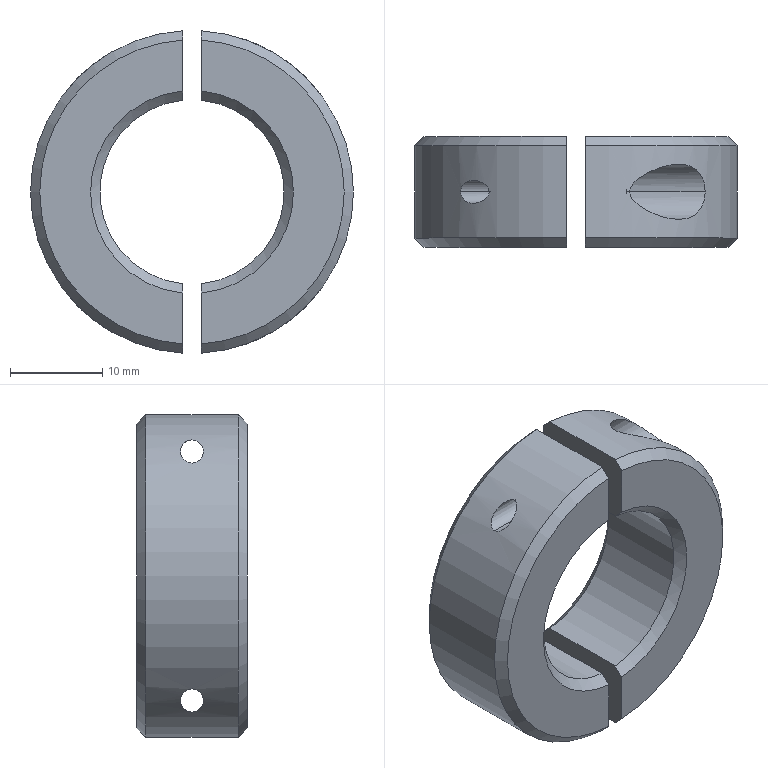Part | SolidWorks | features HoleWzd 2, Chamfer 1, Extrusion 1, ICE 1, MirrorPattern 1 | 2 solids | 34 faces | box 35 x 12 x 34.943 mm | volume 6766 mm3 | cylinder 16 | plane 10 | cone 8 | commonest cylinder face diameters 2.5 x4 3.4 x4 6 x4 20 x2 35 x2
STEP:
#1=CARTESIAN_POINT('',(1.,0.,11.8));
#2=VERTEX_POINT('',#1);
#3=CARTESIAN_POINT('',(1.,0.,15.2));
#4=VERTEX_POINT('',#3);
#5=CARTESIAN_POINT('',(1.,0.,13.5));
#6=DIRECTION('',(1.,0.,0.));
#7=DIRECTION('',(0.,0.,1.));
#8=AXIS2_PLACEMENT_3D('',#5,#6,#7);
#9=CIRCLE('',#8,1.7);
#10=EDGE_CURVE('',#2,#4,#9,.T.);
#11=ORIENTED_EDGE('',*,*,#10,.F.);
#12=CARTESIAN_POINT('',(5.5,0.,11.8));
#13=VERTEX_POINT('',#12);
#14=CARTESIAN_POINT('',(17.5,0.,11.8));
#15=DIRECTION('',(1.,0.,0.));
#16=VECTOR('',#15,1000.);
#17=LINE('',#14,#16);
#18=EDGE_CURVE('',#2,#13,#17,.T.);
#19=ORIENTED_EDGE('',*,*,#18,.T.);
#20=CARTESIAN_POINT('',(5.5,0.,15.2));
#21=VERTEX_POINT('',#20);
#22=CARTESIAN_POINT('',(5.5,0.,13.5));
#23=DIRECTION('',(-1.,0.,0.));
#24=DIRECTION('',(0.,0.,1.));
#25=AXIS2_PLACEMENT_3D('',#22,#23,#24);
#26=CIRCLE('',#25,1.7);
#27=EDGE_CURVE('',#21,#13,#26,.T.);
#28=ORIENTED_EDGE('',*,*,#27,.F.);
#29=CARTESIAN_POINT('',(17.5,0.,15.2));
#30=DIRECTION('',(1.,0.,0.));
#31=VECTOR('',#30,1000.);
#32=LINE('',#29,#31);
#33=EDGE_CURVE('',#4,#21,#32,.T.);
#34=ORIENTED_EDGE('',*,*,#33,.F.);
#35=EDGE_LOOP('',(#11,#19,#28,#34));
#36=FACE_OUTER_BOUND('',#35,.T.);
#37=CARTESIAN_POINT('',(17.5,0.,13.5));
#38=DIRECTION('',(1.,0.,0.));
#39=DIRECTION('',(0.,0.,1.));
#40=AXIS2_PLACEMENT_3D('',#37,#38,#39);
#41=CYLINDRICAL_SURFACE('',#40,1.7);
#42=ADVANCED_FACE('',(#36),#41,.F.);
#43=CARTESIAN_POINT('',(5.5,0.,16.5));
#44=VERTEX_POINT('',#43);
#45=CARTESIAN_POINT('',(5.5,0.,10.5));
#46=VERTEX_POINT('',#45);
#47=CARTESIAN_POINT('',(5.5,0.,13.5));
#48=DIRECTION('',(-1.,0.,0.));
#49=DIRECTION('',(0.,0.,1.));
#50=AXIS2_PLACEMENT_3D('',#47,#48,#49);
#51=CIRCLE('',#50,3.);
#52=EDGE_CURVE('',#44,#46,#51,.T.);
#53=ORIENTED_EDGE('',*,*,#52,.T.);
#54=CARTESIAN_POINT('',(14.,0.,10.5));
#55=VERTEX_POINT('',#54);
#56=CARTESIAN_POINT('',(17.5,0.,10.5));
#57=DIRECTION('',(1.,0.,0.));
#58=VECTOR('',#57,1000.);
#59=LINE('',#56,#58);
#60=EDGE_CURVE('',#46,#55,#59,.T.);
#61=ORIENTED_EDGE('',*,*,#60,.T.);
#62=CARTESIAN_POINT('',(5.831,0.,16.5));
#63=VERTEX_POINT('',#62);
#64=CARTESIAN_POINT('',(14.,0.,10.5));
#65=CARTESIAN_POINT('',(14.,0.273,10.5));
#66=CARTESIAN_POINT('',(13.973,0.5393,10.537));
#67=CARTESIAN_POINT('',(13.864,1.056,10.679));
#68=CARTESIAN_POINT('',(13.786,1.293,10.781));
#69=CARTESIAN_POINT('',(13.582,1.731,11.037));
#70=CARTESIAN_POINT('',(13.461,1.922,11.185));
#71=CARTESIAN_POINT('',(13.183,2.258,11.511));
#72=CARTESIAN_POINT('',(13.03,2.398,11.685));
#73=CARTESIAN_POINT('',(12.701,2.63,12.041));
#74=CARTESIAN_POINT('',(12.523,2.724,12.227));
#75=CARTESIAN_POINT('',(12.154,2.867,12.594));
#76=CARTESIAN_POINT('',(11.963,2.917,12.775));
#77=CARTESIAN_POINT('',(11.569,2.983,13.133));
#78=CARTESIAN_POINT('',(11.364,2.999,13.311));
#79=CARTESIAN_POINT('',(10.948,3.001,13.656));
#80=CARTESIAN_POINT('',(10.737,2.987,13.822));
#81=CARTESIAN_POINT('',(10.099,2.909,14.302));
#82=CARTESIAN_POINT('',(9.664,2.809,14.599));
#83=CARTESIAN_POINT('',(8.778,2.526,15.148));
#84=CARTESIAN_POINT('',(8.336,2.346,15.395));
#85=CARTESIAN_POINT('',(7.683,2.018,15.725));
#86=CARTESIAN_POINT('',(7.466,1.898,15.829));
#87=CARTESIAN_POINT('',(7.041,1.632,16.023));
#88=CARTESIAN_POINT('',(6.83,1.484,16.114));
#89=CARTESIAN_POINT('',(6.434,1.153,16.276));
#90=CARTESIAN_POINT('',(6.246,0.968,16.348));
#91=CARTESIAN_POINT('',(6.02,0.6436,16.432));
#92=CARTESIAN_POINT('',(5.953,0.5249,16.456));
#93=CARTESIAN_POINT('',(5.859,0.2731,16.49));
#94=CARTESIAN_POINT('',(5.831,0.1376,16.5));
#95=CARTESIAN_POINT('',(5.831,0.,16.5));
#96=B_SPLINE_CURVE_WITH_KNOTS('',3,(#64,#65,#66,#67,#68,#69,#70,#71,#72,#73,#74,#75,#76,#77,#78,#79,#80,#81,#82,#83,#84,#85,#86,#87,#88,#89,#90,#91,#92,#93,#94,#95),.UNSPECIFIED.,.F.,.F.,(4,2,2,2,2,2,2,2,2,2,2,2,2,2,2,4),(0.01297,0.01378,0.01459,0.0154,0.01621,0.01702,0.01783,0.01864,0.01945,0.02107,0.02269,0.02351,0.02432,0.02513,0.02553,0.02594),.UNSPECIFIED.);
#97=EDGE_CURVE('',#55,#63,#96,.T.);
#98=ORIENTED_EDGE('',*,*,#97,.T.);
#99=CARTESIAN_POINT('',(17.5,0.,16.5));
#100=DIRECTION('',(1.,0.,0.));
#101=VECTOR('',#100,1000.);
#102=LINE('',#99,#101);
#103=EDGE_CURVE('',#44,#63,#102,.T.);
#104=ORIENTED_EDGE('',*,*,#103,.F.);
#105=EDGE_LOOP('',(#53,#61,#98,#104));
#106=FACE_OUTER_BOUND('',#105,.T.);
#107=CARTESIAN_POINT('',(17.5,0.,13.5));
#108=DIRECTION('',(1.,0.,0.));
#109=DIRECTION('',(0.,0.,1.));
#110=AXIS2_PLACEMENT_3D('',#107,#108,#109);
#111=CYLINDRICAL_SURFACE('',#110,3.);
#112=ADVANCED_FACE('',(#106),#111,.F.);
#113=CARTESIAN_POINT('',(1.,0.,-15.2));
#114=VERTEX_POINT('',#113);
#115=CARTESIAN_POINT('',(1.,0.,-11.8));
#116=VERTEX_POINT('',#115);
#117=CARTESIAN_POINT('',(1.,0.,-13.5));
#118=DIRECTION('',(-1.,0.,0.));
#119=DIRECTION('',(0.,0.,-1.));
#120=AXIS2_PLACEMENT_3D('',#117,#118,#119);
#121=CIRCLE('',#120,1.7);
#122=EDGE_CURVE('',#114,#116,#121,.T.);
#123=ORIENTED_EDGE('',*,*,#122,.T.);
#124=CARTESIAN_POINT('',(5.5,0.,-11.8));
#125=VERTEX_POINT('',#124);
#126=CARTESIAN_POINT('',(17.5,0.,-11.8));
#127=DIRECTION('',(1.,0.,0.));
#128=VECTOR('',#127,1000.);
#129=LINE('',#126,#128);
#130=EDGE_CURVE('',#116,#125,#129,.T.);
#131=ORIENTED_EDGE('',*,*,#130,.T.);
#132=CARTESIAN_POINT('',(5.5,0.,-15.2));
#133=VERTEX_POINT('',#132);
#134=CARTESIAN_POINT('',(5.5,0.,-13.5));
#135=DIRECTION('',(1.,0.,0.));
#136=DIRECTION('',(0.,0.,-1.));
#137=AXIS2_PLACEMENT_3D('',#134,#135,#136);
#138=CIRCLE('',#137,1.7);
#139=EDGE_CURVE('',#125,#133,#138,.T.);
#140=ORIENTED_EDGE('',*,*,#139,.T.);
#141=CARTESIAN_POINT('',(17.5,0.,-15.2));
#142=DIRECTION('',(1.,0.,0.));
#143=VECTOR('',#142,1000.);
#144=LINE('',#141,#143);
#145=EDGE_CURVE('',#114,#133,#144,.T.);
#146=ORIENTED_EDGE('',*,*,#145,.F.);
#147=EDGE_LOOP('',(#123,#131,#140,#146));
#148=FACE_OUTER_BOUND('',#147,.T.);
#149=CARTESIAN_POINT('',(17.5,0.,-13.5));
#150=DIRECTION('',(1.,0.,0.));
#151=DIRECTION('',(0.,0.,-1.));
#152=AXIS2_PLACEMENT_3D('',#149,#150,#151);
#153=CYLINDRICAL_SURFACE('',#152,1.7);
#154=ADVANCED_FACE('',(#148),#153,.F.);
#155=CARTESIAN_POINT('',(5.5,0.,-10.5));
#156=VERTEX_POINT('',#155);
#157=CARTESIAN_POINT('',(5.5,0.,-16.5));
#158=VERTEX_POINT('',#157);
#159=CARTESIAN_POINT('',(5.5,0.,-13.5));
#160=DIRECTION('',(1.,0.,0.));
#161=DIRECTION('',(0.,0.,-1.));
#162=AXIS2_PLACEMENT_3D('',#159,#160,#161);
#163=CIRCLE('',#162,3.);
#164=EDGE_CURVE('',#156,#158,#163,.T.);
#165=ORIENTED_EDGE('',*,*,#164,.F.);
#166=CARTESIAN_POINT('',(14.,0.,-10.5));
#167=VERTEX_POINT('',#166);
#168=CARTESIAN_POINT('',(17.5,0.,-10.5));
#169=DIRECTION('',(1.,0.,0.));
#170=VECTOR('',#169,1000.);
#171=LINE('',#168,#170);
#172=EDGE_CURVE('',#156,#167,#171,.T.);
#173=ORIENTED_EDGE('',*,*,#172,.T.);
#174=CARTESIAN_POINT('',(5.831,0.,-16.5));
#175=VERTEX_POINT('',#174);
#176=CARTESIAN_POINT('',(5.831,0.,-16.5));
#177=CARTESIAN_POINT('',(5.831,-0.1376,-16.5));
#178=CARTESIAN_POINT('',(5.858,-0.2701,-16.491));
#179=CARTESIAN_POINT('',(5.953,-0.5249,-16.457));
#180=CARTESIAN_POINT('',(6.018,-0.641,-16.433));
#181=CARTESIAN_POINT('',(6.17,-0.8592,-16.377));
#182=CARTESIAN_POINT('',(6.256,-0.9603,-16.344));
#183=CARTESIAN_POINT('',(6.437,-1.148,-16.274));
#184=CARTESIAN_POINT('',(6.532,-1.235,-16.236));
#185=CARTESIAN_POINT('',(6.829,-1.483,-16.114));
#186=CARTESIAN_POINT('',(7.039,-1.631,-16.024));
#187=CARTESIAN_POINT('',(7.464,-1.897,-15.83));
#188=CARTESIAN_POINT('',(7.68,-2.017,-15.726));
#189=CARTESIAN_POINT('',(8.335,-2.346,-15.395));
#190=CARTESIAN_POINT('',(8.783,-2.527,-15.145));
#191=CARTESIAN_POINT('',(9.664,-2.808,-14.599));
#192=CARTESIAN_POINT('',(10.098,-2.909,-14.303));
#193=CARTESIAN_POINT('',(10.74,-2.987,-13.819));
#194=CARTESIAN_POINT('',(10.953,-3.001,-13.651));
#195=CARTESIAN_POINT('',(11.368,-2.999,-13.308));
#196=CARTESIAN_POINT('',(11.57,-2.983,-13.132));
#197=CARTESIAN_POINT('',(11.965,-2.916,-12.773));
#198=CARTESIAN_POINT('',(12.159,-2.865,-12.589));
#199=CARTESIAN_POINT('',(12.528,-2.721,-12.222));
#200=CARTESIAN_POINT('',(12.703,-2.629,-12.04));
#201=CARTESIAN_POINT('',(13.032,-2.396,-11.682));
#202=CARTESIAN_POINT('',(13.187,-2.253,-11.506));
#203=CARTESIAN_POINT('',(13.393,-2.004,-11.264));
#204=CARTESIAN_POINT('',(13.458,-1.914,-11.187));
#205=CARTESIAN_POINT('',(13.578,-1.722,-11.04));
#206=CARTESIAN_POINT('',(13.635,-1.618,-10.97));
#207=CARTESIAN_POINT('',(13.735,-1.401,-10.844));
#208=CARTESIAN_POINT('',(13.78,-1.287,-10.787));
#209=CARTESIAN_POINT('',(13.858,-1.049,-10.687));
#210=CARTESIAN_POINT('',(13.892,-0.9236,-10.643));
#211=CARTESIAN_POINT('',(13.973,-0.5391,-10.537));
#212=CARTESIAN_POINT('',(14.,-0.273,-10.5));
#213=CARTESIAN_POINT('',(14.,0.,-10.5));
#214=B_SPLINE_CURVE_WITH_KNOTS('',3,(#176,#177,#178,#179,#180,#181,#182,#183,#184,#185,#186,#187,#188,#189,#190,#191,#192,#193,#194,#195,#196,#197,#198,#199,#200,#201,#202,#203,#204,#205,#206,#207,#208,#209,#210,#211,#212,#213),.UNSPECIFIED.,.F.,.F.,(4,2,2,2,2,2,2,2,2,2,2,2,2,2,2,2,2,2,4),(0.,0.0004053,0.0008105,0.001216,0.001621,0.002432,0.003242,0.004863,0.006484,0.007295,0.008105,0.008916,0.009726,0.01054,0.01094,0.01135,0.01175,0.01216,0.01297),.UNSPECIFIED.);
#215=EDGE_CURVE('',#175,#167,#214,.T.);
#216=ORIENTED_EDGE('',*,*,#215,.F.);
#217=CARTESIAN_POINT('',(17.5,0.,-16.5));
#218=DIRECTION('',(1.,0.,0.));
#219=VECTOR('',#218,1000.);
#220=LINE('',#217,#219);
#221=EDGE_CURVE('',#158,#175,#220,.T.);
#222=ORIENTED_EDGE('',*,*,#221,.F.);
#223=EDGE_LOOP('',(#165,#173,#216,#222));
#224=FACE_OUTER_BOUND('',#223,.T.);
#225=CARTESIAN_POINT('',(17.5,0.,-13.5));
#226=DIRECTION('',(1.,0.,0.));
#227=DIRECTION('',(0.,0.,-1.));
#228=AXIS2_PLACEMENT_3D('',#225,#226,#227);
#229=CYLINDRICAL_SURFACE('',#228,3.);
#230=ADVANCED_FACE('',(#224),#229,.F.);
#231=CARTESIAN_POINT('',(1.,-6.,-10.954));
#232=VERTEX_POINT('',#231);
#233=CARTESIAN_POINT('',(1.,-5.,-9.95));
#234=VERTEX_POINT('',#233);
#235=CARTESIAN_POINT('',(1.,-6.,-10.954));
#236=CARTESIAN_POINT('',(1.,-5.667,-10.62));
#237=CARTESIAN_POINT('',(1.,-5.333,-10.285));
#238=CARTESIAN_POINT('',(1.,-5.,-9.95));
#239=B_SPLINE_CURVE_WITH_KNOTS('',3,(#235,#236,#237,#238),.UNSPECIFIED.,.F.,.F.,(4,4),(0.000000992,0.001418),.UNSPECIFIED.);
#240=EDGE_CURVE('',#232,#234,#239,.T.);
#241=ORIENTED_EDGE('',*,*,#240,.T.);
#242=CARTESIAN_POINT('',(1.,5.,-9.95));
#243=VERTEX_POINT('',#242);
#244=CARTESIAN_POINT('',(1.,6.,-9.95));
#245=DIRECTION('',(0.,1.,0.));
#246=VECTOR('',#245,1000.);
#247=LINE('',#244,#246);
#248=EDGE_CURVE('',#234,#243,#247,.T.);
#249=ORIENTED_EDGE('',*,*,#248,.T.);
#250=CARTESIAN_POINT('',(1.,6.,-10.954));
#251=VERTEX_POINT('',#250);
#252=CARTESIAN_POINT('',(1.,5.,-9.95));
#253=CARTESIAN_POINT('',(1.,5.333,-10.285));
#254=CARTESIAN_POINT('',(1.,5.667,-10.62));
#255=CARTESIAN_POINT('',(1.,6.,-10.954));
#256=B_SPLINE_CURVE_WITH_KNOTS('',3,(#252,#253,#254,#255),.UNSPECIFIED.,.F.,.F.,(4,4),(0.02841,0.02983),.UNSPECIFIED.);
#257=EDGE_CURVE('',#243,#251,#256,.T.);
#258=ORIENTED_EDGE('',*,*,#257,.T.);
#259=CARTESIAN_POINT('',(1.,6.,-16.47));
#260=VERTEX_POINT('',#259);
#261=CARTESIAN_POINT('',(1.,6.,20.));
#262=DIRECTION('',(0.,0.,-1.));
#263=VECTOR('',#262,1000.);
#264=LINE('',#261,#263);
#265=EDGE_CURVE('',#251,#260,#264,.T.);
#266=ORIENTED_EDGE('',*,*,#265,.T.);
#267=CARTESIAN_POINT('',(1.,5.,-17.471));
#268=VERTEX_POINT('',#267);
#269=CARTESIAN_POINT('',(1.,6.,-16.47));
#270=CARTESIAN_POINT('',(1.,5.667,-16.804));
#271=CARTESIAN_POINT('',(1.,5.333,-17.138));
#272=CARTESIAN_POINT('',(1.,5.,-17.471));
#273=B_SPLINE_CURVE_WITH_KNOTS('',3,(#269,#270,#271,#272),.UNSPECIFIED.,.F.,.F.,(4,4),(0.04688,0.0483),.UNSPECIFIED.);
#274=EDGE_CURVE('',#260,#268,#273,.T.);
#275=ORIENTED_EDGE('',*,*,#274,.T.);
#276=CARTESIAN_POINT('',(1.,-5.,-17.471));
#277=VERTEX_POINT('',#276);
#278=CARTESIAN_POINT('',(1.,6.,-17.471));
#279=DIRECTION('',(0.,1.,0.));
#280=VECTOR('',#279,1000.);
#281=LINE('',#278,#280);
#282=EDGE_CURVE('',#277,#268,#281,.T.);
#283=ORIENTED_EDGE('',*,*,#282,.F.);
#284=CARTESIAN_POINT('',(1.,-6.,-16.47));
#285=VERTEX_POINT('',#284);
#286=CARTESIAN_POINT('',(1.,-5.,-17.471));
#287=CARTESIAN_POINT('',(1.,-5.333,-17.138));
#288=CARTESIAN_POINT('',(1.,-5.667,-16.804));
#289=CARTESIAN_POINT('',(1.,-6.,-16.47));
#290=B_SPLINE_CURVE_WITH_KNOTS('',3,(#286,#287,#288,#289),.UNSPECIFIED.,.F.,.F.,(4,4),(0.000000991,0.001416),.UNSPECIFIED.);
#291=EDGE_CURVE('',#277,#285,#290,.T.);
#292=ORIENTED_EDGE('',*,*,#291,.T.);
#293=CARTESIAN_POINT('',(1.,-6.,20.));
#294=DIRECTION('',(0.,0.,-1.));
#295=VECTOR('',#294,1000.);
#296=LINE('',#293,#295);
#297=EDGE_CURVE('',#232,#285,#296,.T.);
#298=ORIENTED_EDGE('',*,*,#297,.F.);
#299=EDGE_LOOP('',(#241,#249,#258,#266,#275,#283,#292,#298));
#300=FACE_OUTER_BOUND('',#299,.T.);
#301=ORIENTED_EDGE('',*,*,#122,.F.);
#302=CARTESIAN_POINT('',(1.,0.,-13.5));
#303=DIRECTION('',(-1.,0.,0.));
#304=DIRECTION('',(0.,0.,-1.));
#305=AXIS2_PLACEMENT_3D('',#302,#303,#304);
#306=CIRCLE('',#305,1.7);
#307=EDGE_CURVE('',#116,#114,#306,.T.);
#308=ORIENTED_EDGE('',*,*,#307,.F.);
#309=EDGE_LOOP('',(#301,#308));
#310=FACE_BOUND('',#309,.T.);
#311=CARTESIAN_POINT('',(1.,-6.,20.));
#312=DIRECTION('',(1.,0.,0.));
#313=DIRECTION('',(0.,0.,-1.));
#314=AXIS2_PLACEMENT_3D('',#311,#312,#313);
#315=PLANE('',#314);
#316=ADVANCED_FACE('',(#300,#310),#315,.F.);
#317=CARTESIAN_POINT('',(1.,6.,16.47));
#318=VERTEX_POINT('',#317);
#319=CARTESIAN_POINT('',(1.,6.,10.954));
#320=VERTEX_POINT('',#319);
#321=CARTESIAN_POINT('',(1.,6.,20.));
#322=DIRECTION('',(0.,0.,-1.));
#323=VECTOR('',#322,1000.);
#324=LINE('',#321,#323);
#325=EDGE_CURVE('',#318,#320,#324,.T.);
#326=ORIENTED_EDGE('',*,*,#325,.F.);
#327=CARTESIAN_POINT('',(0.,6.,0.));
#328=DIRECTION('',(0.,1.,0.));
#329=DIRECTION('',(0.,0.,1.));
#330=AXIS2_PLACEMENT_3D('',#327,#328,#329);
#331=CIRCLE('',#330,16.5);
#332=EDGE_CURVE('',#318,#260,#331,.T.);
#333=ORIENTED_EDGE('',*,*,#332,.T.);
#334=ORIENTED_EDGE('',*,*,#265,.F.);
#335=CARTESIAN_POINT('',(0.,6.,0.));
#336=DIRECTION('',(0.,-1.,0.));
#337=DIRECTION('',(0.,0.,1.));
#338=AXIS2_PLACEMENT_3D('',#335,#336,#337);
#339=CIRCLE('',#338,11.);
#340=EDGE_CURVE('',#251,#320,#339,.T.);
#341=ORIENTED_EDGE('',*,*,#340,.T.);
#342=EDGE_LOOP('',(#326,#333,#334,#341));
#343=FACE_OUTER_BOUND('',#342,.T.);
#344=CARTESIAN_POINT('',(0.,6.,0.));
#345=DIRECTION('',(0.,1.,0.));
#346=DIRECTION('',(0.,0.,1.));
#347=AXIS2_PLACEMENT_3D('',#344,#345,#346);
#348=PLANE('',#347);
#349=ADVANCED_FACE('',(#343),#348,.T.);
#350=CARTESIAN_POINT('',(1.,-6.,16.47));
#351=VERTEX_POINT('',#350);
#352=CARTESIAN_POINT('',(0.,-6.,0.));
#353=DIRECTION('',(0.,-1.,0.));
#354=DIRECTION('',(0.,0.,1.));
#355=AXIS2_PLACEMENT_3D('',#352,#353,#354);
#356=CIRCLE('',#355,16.5);
#357=EDGE_CURVE('',#285,#351,#356,.T.);
#358=ORIENTED_EDGE('',*,*,#357,.T.);
#359=CARTESIAN_POINT('',(1.,-6.,10.954));
#360=VERTEX_POINT('',#359);
#361=CARTESIAN_POINT('',(1.,-6.,20.));
#362=DIRECTION('',(0.,0.,-1.));
#363=VECTOR('',#362,1000.);
#364=LINE('',#361,#363);
#365=EDGE_CURVE('',#351,#360,#364,.T.);
#366=ORIENTED_EDGE('',*,*,#365,.T.);
#367=CARTESIAN_POINT('',(0.,-6.,0.));
#368=DIRECTION('',(0.,1.,0.));
#369=DIRECTION('',(0.,0.,1.));
#370=AXIS2_PLACEMENT_3D('',#367,#368,#369);
#371=CIRCLE('',#370,11.);
#372=EDGE_CURVE('',#360,#232,#371,.T.);
#373=ORIENTED_EDGE('',*,*,#372,.T.);
#374=ORIENTED_EDGE('',*,*,#297,.T.);
#375=EDGE_LOOP('',(#358,#366,#373,#374));
#376=FACE_OUTER_BOUND('',#375,.T.);
#377=CARTESIAN_POINT('',(0.,-6.,0.));
#378=DIRECTION('',(0.,1.,0.));
#379=DIRECTION('',(0.,0.,1.));
#380=AXIS2_PLACEMENT_3D('',#377,#378,#379);
#381=PLANE('',#380);
#382=ADVANCED_FACE('',(#376),#381,.F.);
#383=CARTESIAN_POINT('',(5.831,0.,16.5));
#384=CARTESIAN_POINT('',(5.831,-0.1376,16.5));
#385=CARTESIAN_POINT('',(5.858,-0.2701,16.491));
#386=CARTESIAN_POINT('',(5.953,-0.5249,16.457));
#387=CARTESIAN_POINT('',(6.018,-0.641,16.433));
#388=CARTESIAN_POINT('',(6.17,-0.8592,16.377));
#389=CARTESIAN_POINT('',(6.256,-0.9603,16.344));
#390=CARTESIAN_POINT('',(6.437,-1.148,16.274));
#391=CARTESIAN_POINT('',(6.532,-1.235,16.236));
#392=CARTESIAN_POINT('',(6.829,-1.483,16.114));
#393=CARTESIAN_POINT('',(7.039,-1.631,16.024));
#394=CARTESIAN_POINT('',(7.464,-1.897,15.83));
#395=CARTESIAN_POINT('',(7.68,-2.017,15.726));
#396=CARTESIAN_POINT('',(8.335,-2.346,15.395));
#397=CARTESIAN_POINT('',(8.783,-2.527,15.145));
#398=CARTESIAN_POINT('',(9.664,-2.808,14.599));
#399=CARTESIAN_POINT('',(10.098,-2.909,14.303));
#400=CARTESIAN_POINT('',(10.74,-2.987,13.819));
#401=CARTESIAN_POINT('',(10.953,-3.001,13.651));
#402=CARTESIAN_POINT('',(11.368,-2.999,13.308));
#403=CARTESIAN_POINT('',(11.57,-2.983,13.132));
#404=CARTESIAN_POINT('',(11.965,-2.916,12.773));
#405=CARTESIAN_POINT('',(12.159,-2.865,12.589));
#406=CARTESIAN_POINT('',(12.528,-2.721,12.222));
#407=CARTESIAN_POINT('',(12.703,-2.629,12.04));
#408=CARTESIAN_POINT('',(13.032,-2.396,11.682));
#409=CARTESIAN_POINT('',(13.187,-2.253,11.506));
#410=CARTESIAN_POINT('',(13.393,-2.004,11.264));
#411=CARTESIAN_POINT('',(13.458,-1.914,11.187));
#412=CARTESIAN_POINT('',(13.578,-1.722,11.04));
#413=CARTESIAN_POINT('',(13.635,-1.618,10.97));
#414=CARTESIAN_POINT('',(13.735,-1.401,10.844));
#415=CARTESIAN_POINT('',(13.78,-1.287,10.787));
#416=CARTESIAN_POINT('',(13.858,-1.049,10.687));
#417=CARTESIAN_POINT('',(13.892,-0.9236,10.643));
#418=CARTESIAN_POINT('',(13.973,-0.5391,10.537));
#419=CARTESIAN_POINT('',(14.,-0.273,10.5));
#420=CARTESIAN_POINT('',(14.,0.,10.5));
#421=B_SPLINE_CURVE_WITH_KNOTS('',3,(#383,#384,#385,#386,#387,#388,#389,#390,#391,#392,#393,#394,#395,#396,#397,#398,#399,#400,#401,#402,#403,#404,#405,#406,#407,#408,#409,#410,#411,#412,#413,#414,#415,#416,#417,#418,#419,#420),.UNSPECIFIED.,.F.,.F.,(4,2,2,2,2,2,2,2,2,2,2,2,2,2,2,2,2,2,4),(0.,0.0004053,0.0008105,0.001216,0.001621,0.002432,0.003242,0.004863,0.006484,0.007295,0.008105,0.008916,0.009726,0.01054,0.01094,0.01135,0.01175,0.01216,0.01297),.UNSPECIFIED.);
#422=EDGE_CURVE('',#63,#55,#421,.T.);
#423=ORIENTED_EDGE('',*,*,#422,.F.);
#424=ORIENTED_EDGE('',*,*,#97,.F.);
#425=EDGE_LOOP('',(#423,#424));
#426=FACE_BOUND('',#425,.T.);
#427=ORIENTED_EDGE('',*,*,#215,.T.);
#428=CARTESIAN_POINT('',(14.,0.,-10.5));
#429=CARTESIAN_POINT('',(14.,0.273,-10.5));
#430=CARTESIAN_POINT('',(13.973,0.5393,-10.537));
#431=CARTESIAN_POINT('',(13.864,1.056,-10.679));
#432=CARTESIAN_POINT('',(13.786,1.293,-10.781));
#433=CARTESIAN_POINT('',(13.582,1.731,-11.037));
#434=CARTESIAN_POINT('',(13.461,1.922,-11.185));
#435=CARTESIAN_POINT('',(13.183,2.258,-11.511));
#436=CARTESIAN_POINT('',(13.03,2.398,-11.685));
#437=CARTESIAN_POINT('',(12.701,2.63,-12.041));
#438=CARTESIAN_POINT('',(12.523,2.724,-12.227));
#439=CARTESIAN_POINT('',(12.154,2.867,-12.594));
#440=CARTESIAN_POINT('',(11.963,2.917,-12.775));
#441=CARTESIAN_POINT('',(11.569,2.983,-13.133));
#442=CARTESIAN_POINT('',(11.364,2.999,-13.311));
#443=CARTESIAN_POINT('',(10.948,3.001,-13.656));
#444=CARTESIAN_POINT('',(10.737,2.987,-13.822));
#445=CARTESIAN_POINT('',(10.099,2.909,-14.302));
#446=CARTESIAN_POINT('',(9.664,2.809,-14.599));
#447=CARTESIAN_POINT('',(8.778,2.526,-15.148));
#448=CARTESIAN_POINT('',(8.336,2.346,-15.395));
#449=CARTESIAN_POINT('',(7.683,2.018,-15.725));
#450=CARTESIAN_POINT('',(7.466,1.898,-15.829));
#451=CARTESIAN_POINT('',(7.041,1.632,-16.023));
#452=CARTESIAN_POINT('',(6.83,1.484,-16.114));
#453=CARTESIAN_POINT('',(6.434,1.153,-16.276));
#454=CARTESIAN_POINT('',(6.246,0.968,-16.348));
#455=CARTESIAN_POINT('',(6.02,0.6436,-16.432));
#456=CARTESIAN_POINT('',(5.953,0.5249,-16.456));
#457=CARTESIAN_POINT('',(5.859,0.2731,-16.49));
#458=CARTESIAN_POINT('',(5.831,0.1376,-16.5));
#459=CARTESIAN_POINT('',(5.831,0.,-16.5));
#460=B_SPLINE_CURVE_WITH_KNOTS('',3,(#428,#429,#430,#431,#432,#433,#434,#435,#436,#437,#438,#439,#440,#441,#442,#443,#444,#445,#446,#447,#448,#449,#450,#451,#452,#453,#454,#455,#456,#457,#458,#459),.UNSPECIFIED.,.F.,.F.,(4,2,2,2,2,2,2,2,2,2,2,2,2,2,2,4),(0.01297,0.01378,0.01459,0.0154,0.01621,0.01702,0.01783,0.01864,0.01945,0.02107,0.02269,0.02351,0.02432,0.02513,0.02553,0.02594),.UNSPECIFIED.);
#461=EDGE_CURVE('',#167,#175,#460,.T.);
#462=ORIENTED_EDGE('',*,*,#461,.T.);
#463=EDGE_LOOP('',(#427,#462));
#464=FACE_BOUND('',#463,.T.);
#465=CARTESIAN_POINT('',(1.,5.,17.471));
#466=VERTEX_POINT('',#465);
#467=CARTESIAN_POINT('',(0.,5.,0.));
#468=DIRECTION('',(0.,-1.,0.));
#469=DIRECTION('',(0.,0.,1.));
#470=AXIS2_PLACEMENT_3D('',#467,#468,#469);
#471=CIRCLE('',#470,17.5);
#472=EDGE_CURVE('',#268,#466,#471,.T.);
#473=ORIENTED_EDGE('',*,*,#472,.T.);
#474=CARTESIAN_POINT('',(1.,-5.,17.471));
#475=VERTEX_POINT('',#474);
#476=CARTESIAN_POINT('',(1.,6.,17.471));
#477=DIRECTION('',(0.,-1.,0.));
#478=VECTOR('',#477,1000.);
#479=LINE('',#476,#478);
#480=EDGE_CURVE('',#466,#475,#479,.T.);
#481=ORIENTED_EDGE('',*,*,#480,.T.);
#482=CARTESIAN_POINT('',(0.,-5.,0.));
#483=DIRECTION('',(0.,1.,0.));
#484=DIRECTION('',(0.,0.,1.));
#485=AXIS2_PLACEMENT_3D('',#482,#483,#484);
#486=CIRCLE('',#485,17.5);
#487=EDGE_CURVE('',#475,#277,#486,.T.);
#488=ORIENTED_EDGE('',*,*,#487,.T.);
#489=ORIENTED_EDGE('',*,*,#282,.T.);
#490=EDGE_LOOP('',(#473,#481,#488,#489));
#491=FACE_OUTER_BOUND('',#490,.T.);
#492=CARTESIAN_POINT('',(0.,6.,0.));
#493=DIRECTION('',(0.,-1.,0.));
#494=DIRECTION('',(0.,0.,-1.));
#495=AXIS2_PLACEMENT_3D('',#492,#493,#494);
#496=CYLINDRICAL_SURFACE('',#495,17.5);
#497=ADVANCED_FACE('',(#426,#464,#491),#496,.T.);
#498=CARTESIAN_POINT('',(1.,5.,9.95));
#499=VERTEX_POINT('',#498);
#500=CARTESIAN_POINT('',(1.,-5.,9.95));
#501=VERTEX_POINT('',#500);
#502=CARTESIAN_POINT('',(1.,6.,9.95));
#503=DIRECTION('',(0.,-1.,0.));
#504=VECTOR('',#503,1000.);
#505=LINE('',#502,#504);
#506=EDGE_CURVE('',#499,#501,#505,.T.);
#507=ORIENTED_EDGE('',*,*,#506,.F.);
#508=CARTESIAN_POINT('',(0.,5.,0.));
#509=DIRECTION('',(0.,1.,0.));
#510=DIRECTION('',(0.,0.,1.));
#511=AXIS2_PLACEMENT_3D('',#508,#509,#510);
#512=CIRCLE('',#511,10.);
#513=EDGE_CURVE('',#499,#243,#512,.T.);
#514=ORIENTED_EDGE('',*,*,#513,.T.);
#515=ORIENTED_EDGE('',*,*,#248,.F.);
#516=CARTESIAN_POINT('',(0.,-5.,0.));
#517=DIRECTION('',(0.,-1.,0.));
#518=DIRECTION('',(0.,0.,1.));
#519=AXIS2_PLACEMENT_3D('',#516,#517,#518);
#520=CIRCLE('',#519,10.);
#521=EDGE_CURVE('',#234,#501,#520,.T.);
#522=ORIENTED_EDGE('',*,*,#521,.T.);
#523=EDGE_LOOP('',(#507,#514,#515,#522));
#524=FACE_OUTER_BOUND('',#523,.T.);
#525=CARTESIAN_POINT('',(0.,6.,0.));
#526=DIRECTION('',(0.,-1.,0.));
#527=DIRECTION('',(0.,0.,-1.));
#528=AXIS2_PLACEMENT_3D('',#525,#526,#527);
#529=CYLINDRICAL_SURFACE('',#528,10.);
#530=ADVANCED_FACE('',(#524),#529,.F.);
#531=ORIENTED_EDGE('',*,*,#240,.F.);
#532=ORIENTED_EDGE('',*,*,#372,.F.);
#533=CARTESIAN_POINT('',(1.,-5.,9.95));
#534=CARTESIAN_POINT('',(1.,-5.333,10.285));
#535=CARTESIAN_POINT('',(1.,-5.667,10.62));
#536=CARTESIAN_POINT('',(1.,-6.,10.954));
#537=B_SPLINE_CURVE_WITH_KNOTS('',3,(#533,#534,#535,#536),.UNSPECIFIED.,.F.,.F.,(4,4),(0.02841,0.02983),.UNSPECIFIED.);
#538=EDGE_CURVE('',#501,#360,#537,.T.);
#539=ORIENTED_EDGE('',*,*,#538,.F.);
#540=ORIENTED_EDGE('',*,*,#521,.F.);
#541=EDGE_LOOP('',(#531,#532,#539,#540));
#542=FACE_OUTER_BOUND('',#541,.T.);
#543=CARTESIAN_POINT('',(0.,-6.,0.));
#544=DIRECTION('',(0.,-1.,0.));
#545=DIRECTION('',(0.,0.,-1.));
#546=AXIS2_PLACEMENT_3D('',#543,#544,#545);
#547=CONICAL_SURFACE('',#546,11.,0.7854);
#548=ADVANCED_FACE('',(#542),#547,.F.);
#549=ORIENTED_EDGE('',*,*,#291,.F.);
#550=ORIENTED_EDGE('',*,*,#487,.F.);
#551=CARTESIAN_POINT('',(1.,-6.,16.47));
#552=CARTESIAN_POINT('',(1.,-5.667,16.804));
#553=CARTESIAN_POINT('',(1.,-5.333,17.138));
#554=CARTESIAN_POINT('',(1.,-5.,17.471));
#555=B_SPLINE_CURVE_WITH_KNOTS('',3,(#551,#552,#553,#554),.UNSPECIFIED.,.F.,.F.,(4,4),(0.04688,0.0483),.UNSPECIFIED.);
#556=EDGE_CURVE('',#351,#475,#555,.T.);
#557=ORIENTED_EDGE('',*,*,#556,.F.);
#558=ORIENTED_EDGE('',*,*,#357,.F.);
#559=EDGE_LOOP('',(#549,#550,#557,#558));
#560=FACE_OUTER_BOUND('',#559,.T.);
#561=CARTESIAN_POINT('',(0.,-5.,0.));
#562=DIRECTION('',(0.,1.,0.));
#563=DIRECTION('',(0.,0.,1.));
#564=AXIS2_PLACEMENT_3D('',#561,#562,#563);
#565=CONICAL_SURFACE('',#564,17.5,0.7854);
#566=ADVANCED_FACE('',(#560),#565,.T.);
#567=CARTESIAN_POINT('',(1.,6.,10.954));
#568=CARTESIAN_POINT('',(1.,5.667,10.62));
#569=CARTESIAN_POINT('',(1.,5.333,10.285));
#570=CARTESIAN_POINT('',(1.,5.,9.95));
#571=B_SPLINE_CURVE_WITH_KNOTS('',3,(#567,#568,#569,#570),.UNSPECIFIED.,.F.,.F.,(4,4),(0.000000992,0.001418),.UNSPECIFIED.);
#572=EDGE_CURVE('',#320,#499,#571,.T.);
#573=ORIENTED_EDGE('',*,*,#572,.F.);
#574=ORIENTED_EDGE('',*,*,#340,.F.);
#575=ORIENTED_EDGE('',*,*,#257,.F.);
#576=ORIENTED_EDGE('',*,*,#513,.F.);
#577=EDGE_LOOP('',(#573,#574,#575,#576));
#578=FACE_OUTER_BOUND('',#577,.T.);
#579=CARTESIAN_POINT('',(0.,5.,0.));
#580=DIRECTION('',(0.,1.,0.));
#581=DIRECTION('',(0.,0.,1.));
#582=AXIS2_PLACEMENT_3D('',#579,#580,#581);
#583=CONICAL_SURFACE('',#582,10.,0.7854);
#584=ADVANCED_FACE('',(#578),#583,.F.);
#585=CARTESIAN_POINT('',(1.,5.,17.471));
#586=CARTESIAN_POINT('',(1.,5.333,17.138));
#587=CARTESIAN_POINT('',(1.,5.667,16.804));
#588=CARTESIAN_POINT('',(1.,6.,16.47));
#589=B_SPLINE_CURVE_WITH_KNOTS('',3,(#585,#586,#587,#588),.UNSPECIFIED.,.F.,.F.,(4,4),(0.000000991,0.001416),.UNSPECIFIED.);
#590=EDGE_CURVE('',#466,#318,#589,.T.);
#591=ORIENTED_EDGE('',*,*,#590,.F.);
#592=ORIENTED_EDGE('',*,*,#472,.F.);
#593=ORIENTED_EDGE('',*,*,#274,.F.);
#594=ORIENTED_EDGE('',*,*,#332,.F.);
#595=EDGE_LOOP('',(#591,#592,#593,#594));
#596=FACE_OUTER_BOUND('',#595,.T.);
#597=CARTESIAN_POINT('',(0.,6.,0.));
#598=DIRECTION('',(0.,-1.,0.));
#599=DIRECTION('',(0.,0.,-1.));
#600=AXIS2_PLACEMENT_3D('',#597,#598,#599);
#601=CONICAL_SURFACE('',#600,16.5,0.7854);
#602=ADVANCED_FACE('',(#596),#601,.T.);
#603=CARTESIAN_POINT('',(1.,0.,13.5));
#604=DIRECTION('',(1.,0.,0.));
#605=DIRECTION('',(0.,0.,1.));
#606=AXIS2_PLACEMENT_3D('',#603,#604,#605);
#607=CIRCLE('',#606,1.7);
#608=EDGE_CURVE('',#4,#2,#607,.T.);
#609=ORIENTED_EDGE('',*,*,#608,.T.);
#610=ORIENTED_EDGE('',*,*,#10,.T.);
#611=EDGE_LOOP('',(#609,#610));
#612=FACE_BOUND('',#611,.T.);
#613=ORIENTED_EDGE('',*,*,#538,.T.);
#614=ORIENTED_EDGE('',*,*,#365,.F.);
#615=ORIENTED_EDGE('',*,*,#556,.T.);
#616=ORIENTED_EDGE('',*,*,#480,.F.);
#617=ORIENTED_EDGE('',*,*,#590,.T.);
#618=ORIENTED_EDGE('',*,*,#325,.T.);
#619=ORIENTED_EDGE('',*,*,#572,.T.);
#620=ORIENTED_EDGE('',*,*,#506,.T.);
#621=EDGE_LOOP('',(#613,#614,#615,#616,#617,#618,#619,#620));
#622=FACE_OUTER_BOUND('',#621,.T.);
#623=CARTESIAN_POINT('',(1.,-6.,20.));
#624=DIRECTION('',(1.,0.,0.));
#625=DIRECTION('',(0.,0.,-1.));
#626=AXIS2_PLACEMENT_3D('',#623,#624,#625);
#627=PLANE('',#626);
#628=ADVANCED_FACE('',(#612,#622),#627,.F.);
#629=ORIENTED_EDGE('',*,*,#172,.F.);
#630=CARTESIAN_POINT('',(5.5,0.,-13.5));
#631=DIRECTION('',(1.,0.,0.));
#632=DIRECTION('',(0.,0.,-1.));
#633=AXIS2_PLACEMENT_3D('',#630,#631,#632);
#634=CIRCLE('',#633,3.);
#635=EDGE_CURVE('',#158,#156,#634,.T.);
#636=ORIENTED_EDGE('',*,*,#635,.F.);
#637=ORIENTED_EDGE('',*,*,#221,.T.);
#638=ORIENTED_EDGE('',*,*,#461,.F.);
#639=EDGE_LOOP('',(#629,#636,#637,#638));
#640=FACE_OUTER_BOUND('',#639,.T.);
#641=CARTESIAN_POINT('',(17.5,0.,-13.5));
#642=DIRECTION('',(1.,0.,0.));
#643=DIRECTION('',(0.,0.,-1.));
#644=AXIS2_PLACEMENT_3D('',#641,#642,#643);
#645=CYLINDRICAL_SURFACE('',#644,3.);
#646=ADVANCED_FACE('',(#640),#645,.F.);
#647=ORIENTED_EDGE('',*,*,#130,.F.);
#648=ORIENTED_EDGE('',*,*,#307,.T.);
#649=ORIENTED_EDGE('',*,*,#145,.T.);
#650=CARTESIAN_POINT('',(5.5,0.,-13.5));
#651=DIRECTION('',(1.,0.,0.));
#652=DIRECTION('',(0.,0.,-1.));
#653=AXIS2_PLACEMENT_3D('',#650,#651,#652);
#654=CIRCLE('',#653,1.7);
#655=EDGE_CURVE('',#133,#125,#654,.T.);
#656=ORIENTED_EDGE('',*,*,#655,.T.);
#657=EDGE_LOOP('',(#647,#648,#649,#656));
#658=FACE_OUTER_BOUND('',#657,.T.);
#659=CARTESIAN_POINT('',(17.5,0.,-13.5));
#660=DIRECTION('',(1.,0.,0.));
#661=DIRECTION('',(0.,0.,-1.));
#662=AXIS2_PLACEMENT_3D('',#659,#660,#661);
#663=CYLINDRICAL_SURFACE('',#662,1.7);
#664=ADVANCED_FACE('',(#658),#663,.F.);
#665=ORIENTED_EDGE('',*,*,#655,.F.);
#666=ORIENTED_EDGE('',*,*,#139,.F.);
#667=EDGE_LOOP('',(#665,#666));
#668=FACE_BOUND('',#667,.T.);
#669=ORIENTED_EDGE('',*,*,#635,.T.);
#670=ORIENTED_EDGE('',*,*,#164,.T.);
#671=EDGE_LOOP('',(#669,#670));
#672=FACE_OUTER_BOUND('',#671,.T.);
#673=CARTESIAN_POINT('',(5.5,1.7,-13.5));
#674=DIRECTION('',(-1.,0.,0.));
#675=DIRECTION('',(0.,0.,1.));
#676=AXIS2_PLACEMENT_3D('',#673,#674,#675);
#677=PLANE('',#676);
#678=ADVANCED_FACE('',(#668,#672),#677,.F.);
#679=ORIENTED_EDGE('',*,*,#60,.F.);
#680=CARTESIAN_POINT('',(5.5,0.,13.5));
#681=DIRECTION('',(-1.,0.,0.));
#682=DIRECTION('',(0.,0.,1.));
#683=AXIS2_PLACEMENT_3D('',#680,#681,#682);
#684=CIRCLE('',#683,3.);
#685=EDGE_CURVE('',#46,#44,#684,.T.);
#686=ORIENTED_EDGE('',*,*,#685,.T.);
#687=ORIENTED_EDGE('',*,*,#103,.T.);
#688=ORIENTED_EDGE('',*,*,#422,.T.);
#689=EDGE_LOOP('',(#679,#686,#687,#688));
#690=FACE_OUTER_BOUND('',#689,.T.);
#691=CARTESIAN_POINT('',(17.5,0.,13.5));
#692=DIRECTION('',(1.,0.,0.));
#693=DIRECTION('',(0.,0.,1.));
#694=AXIS2_PLACEMENT_3D('',#691,#692,#693);
#695=CYLINDRICAL_SURFACE('',#694,3.);
#696=ADVANCED_FACE('',(#690),#695,.F.);
#697=ORIENTED_EDGE('',*,*,#18,.F.);
#698=ORIENTED_EDGE('',*,*,#608,.F.);
#699=ORIENTED_EDGE('',*,*,#33,.T.);
#700=CARTESIAN_POINT('',(5.5,0.,13.5));
#701=DIRECTION('',(-1.,0.,0.));
#702=DIRECTION('',(0.,0.,1.));
#703=AXIS2_PLACEMENT_3D('',#700,#701,#702);
#704=CIRCLE('',#703,1.7);
#705=EDGE_CURVE('',#13,#21,#704,.T.);
#706=ORIENTED_EDGE('',*,*,#705,.F.);
#707=EDGE_LOOP('',(#697,#698,#699,#706));
#708=FACE_OUTER_BOUND('',#707,.T.);
#709=CARTESIAN_POINT('',(17.5,0.,13.5));
#710=DIRECTION('',(1.,0.,0.));
#711=DIRECTION('',(0.,0.,1.));
#712=AXIS2_PLACEMENT_3D('',#709,#710,#711);
#713=CYLINDRICAL_SURFACE('',#712,1.7);
#714=ADVANCED_FACE('',(#708),#713,.F.);
#715=ORIENTED_EDGE('',*,*,#27,.T.);
#716=ORIENTED_EDGE('',*,*,#705,.T.);
#717=EDGE_LOOP('',(#715,#716));
#718=FACE_BOUND('',#717,.T.);
#719=ORIENTED_EDGE('',*,*,#52,.F.);
#720=ORIENTED_EDGE('',*,*,#685,.F.);
#721=EDGE_LOOP('',(#719,#720));
#722=FACE_OUTER_BOUND('',#721,.T.);
#723=CARTESIAN_POINT('',(5.5,1.7,13.5));
#724=DIRECTION('',(-1.,0.,0.));
#725=DIRECTION('',(0.,0.,-1.));
#726=AXIS2_PLACEMENT_3D('',#723,#724,#725);
#727=PLANE('',#726);
#728=ADVANCED_FACE('',(#718,#722),#727,.F.);
#729=CLOSED_SHELL('',(#42,#112,#154,#230,#316,#349,#382,#497,#530,#548,#566,#584,#602,#628,#646,#664,#678,#696,#714,#728));
#730=MANIFOLD_SOLID_BREP('',#729);
#731=CARTESIAN_POINT('',(-9.417,0.,14.75));
#732=VERTEX_POINT('',#731);
#733=CARTESIAN_POINT('',(-12.497,0.,12.25));
#734=VERTEX_POINT('',#733);
#735=CARTESIAN_POINT('',(-9.417,0.,14.75));
#736=CARTESIAN_POINT('',(-9.417,0.1092,14.75));
#737=CARTESIAN_POINT('',(-9.44,0.2158,14.735));
#738=CARTESIAN_POINT('',(-9.518,0.4101,14.685));
#739=CARTESIAN_POINT('',(-9.573,0.4984,14.65));
#740=CARTESIAN_POINT('',(-9.758,0.7327,14.528));
#741=CARTESIAN_POINT('',(-9.91,0.853,14.425));
#742=CARTESIAN_POINT('',(-10.222,1.042,14.205));
#743=CARTESIAN_POINT('',(-10.388,1.113,14.085));
#744=CARTESIAN_POINT('',(-10.72,1.212,13.834));
#745=CARTESIAN_POINT('',(-10.886,1.241,13.704));
#746=CARTESIAN_POINT('',(-11.216,1.256,13.435));
#747=CARTESIAN_POINT('',(-11.382,1.241,13.295));
#748=CARTESIAN_POINT('',(-11.697,1.162,13.018));
#749=CARTESIAN_POINT('',(-11.85,1.097,12.878));
#750=CARTESIAN_POINT('',(-12.128,0.9004,12.618));
#751=CARTESIAN_POINT('',(-12.254,0.7677,12.495));
#752=CARTESIAN_POINT('',(-12.393,0.5121,12.356));
#753=CARTESIAN_POINT('',(-12.431,0.4171,12.317));
#754=CARTESIAN_POINT('',(-12.484,0.2153,12.264));
#755=CARTESIAN_POINT('',(-12.497,0.1072,12.25));
#756=CARTESIAN_POINT('',(-12.497,0.,12.25));
#757=B_SPLINE_CURVE_WITH_KNOTS('',3,(#735,#736,#737,#738,#739,#740,#741,#742,#743,#744,#745,#746,#747,#748,#749,#750,#751,#752,#753,#754,#755,#756),.UNSPECIFIED.,.F.,.F.,(4,2,2,2,2,2,2,2,2,2,4),(0.,0.0003224,0.0006448,0.00129,0.001934,0.002579,0.003224,0.003869,0.004514,0.004836,0.005158),.UNSPECIFIED.);
#758=EDGE_CURVE('',#732,#734,#757,.T.);
#759=ORIENTED_EDGE('',*,*,#758,.T.);
#760=CARTESIAN_POINT('',(-1.,0.,12.25));
#761=VERTEX_POINT('',#760);
#762=CARTESIAN_POINT('',(-1.,0.,12.25));
#763=DIRECTION('',(1.,0.,0.));
#764=VECTOR('',#763,1000.);
#765=LINE('',#762,#764);
#766=EDGE_CURVE('',#734,#761,#765,.T.);
#767=ORIENTED_EDGE('',*,*,#766,.T.);
#768=CARTESIAN_POINT('',(-1.,0.,14.75));
#769=VERTEX_POINT('',#768);
#770=CARTESIAN_POINT('',(-1.,0.,13.5));
#771=DIRECTION('',(-1.,0.,0.));
#772=DIRECTION('',(0.,0.,1.));
#773=AXIS2_PLACEMENT_3D('',#770,#771,#772);
#774=CIRCLE('',#773,1.25);
#775=EDGE_CURVE('',#769,#761,#774,.T.);
#776=ORIENTED_EDGE('',*,*,#775,.F.);
#777=CARTESIAN_POINT('',(-1.,0.,14.75));
#778=DIRECTION('',(1.,0.,0.));
#779=VECTOR('',#778,1000.);
#780=LINE('',#777,#779);
#781=EDGE_CURVE('',#732,#769,#780,.T.);
#782=ORIENTED_EDGE('',*,*,#781,.F.);
#783=EDGE_LOOP('',(#759,#767,#776,#782));
#784=FACE_OUTER_BOUND('',#783,.T.);
#785=CARTESIAN_POINT('',(-1.,0.,13.5));
#786=DIRECTION('',(1.,0.,0.));
#787=DIRECTION('',(0.,0.,1.));
#788=AXIS2_PLACEMENT_3D('',#785,#786,#787);
#789=CYLINDRICAL_SURFACE('',#788,1.25);
#790=ADVANCED_FACE('',(#784),#789,.F.);
#791=CARTESIAN_POINT('',(-12.497,0.,-12.25));
#792=VERTEX_POINT('',#791);
#793=CARTESIAN_POINT('',(-9.417,0.,-14.75));
#794=VERTEX_POINT('',#793);
#795=CARTESIAN_POINT('',(-12.497,0.,-12.25));
#796=CARTESIAN_POINT('',(-12.497,-0.1072,-12.25));
#797=CARTESIAN_POINT('',(-12.484,-0.2155,-12.264));
#798=CARTESIAN_POINT('',(-12.431,-0.4175,-12.317));
#799=CARTESIAN_POINT('',(-12.393,-0.5126,-12.356));
#800=CARTESIAN_POINT('',(-12.253,-0.7686,-12.495));
#801=CARTESIAN_POINT('',(-12.127,-0.9009,-12.618));
#802=CARTESIAN_POINT('',(-11.849,-1.098,-12.88));
#803=CARTESIAN_POINT('',(-11.697,-1.162,-13.018));
#804=CARTESIAN_POINT('',(-11.379,-1.242,-13.297));
#805=CARTESIAN_POINT('',(-11.217,-1.255,-13.434));
#806=CARTESIAN_POINT('',(-10.887,-1.241,-13.703));
#807=CARTESIAN_POINT('',(-10.718,-1.212,-13.836));
#808=CARTESIAN_POINT('',(-10.388,-1.113,-14.085));
#809=CARTESIAN_POINT('',(-10.225,-1.044,-14.204));
#810=CARTESIAN_POINT('',(-9.987,-0.9,-14.371));
#811=CARTESIAN_POINT('',(-9.911,-0.8463,-14.423));
#812=CARTESIAN_POINT('',(-9.765,-0.7235,-14.522));
#813=CARTESIAN_POINT('',(-9.695,-0.654,-14.569));
#814=CARTESIAN_POINT('',(-9.573,-0.4982,-14.65));
#815=CARTESIAN_POINT('',(-9.518,-0.4099,-14.685));
#816=CARTESIAN_POINT('',(-9.441,-0.216,-14.735));
#817=CARTESIAN_POINT('',(-9.417,-0.1091,-14.75));
#818=CARTESIAN_POINT('',(-9.417,0.,-14.75));
#819=B_SPLINE_CURVE_WITH_KNOTS('',3,(#795,#796,#797,#798,#799,#800,#801,#802,#803,#804,#805,#806,#807,#808,#809,#810,#811,#812,#813,#814,#815,#816,#817,#818),.UNSPECIFIED.,.F.,.F.,(4,2,2,2,2,2,2,2,2,2,2,4),(0.005158,0.005481,0.005803,0.006447,0.007092,0.007736,0.008381,0.009025,0.009347,0.00967,0.009992,0.01031),.UNSPECIFIED.);
#820=EDGE_CURVE('',#792,#794,#819,.T.);
#821=ORIENTED_EDGE('',*,*,#820,.F.);
#822=CARTESIAN_POINT('',(-1.,0.,-12.25));
#823=VERTEX_POINT('',#822);
#824=CARTESIAN_POINT('',(-1.,0.,-12.25));
#825=DIRECTION('',(1.,0.,0.));
#826=VECTOR('',#825,1000.);
#827=LINE('',#824,#826);
#828=EDGE_CURVE('',#792,#823,#827,.T.);
#829=ORIENTED_EDGE('',*,*,#828,.T.);
#830=CARTESIAN_POINT('',(-1.,0.,-14.75));
#831=VERTEX_POINT('',#830);
#832=CARTESIAN_POINT('',(-1.,0.,-13.5));
#833=DIRECTION('',(1.,0.,0.));
#834=DIRECTION('',(0.,0.,-1.));
#835=AXIS2_PLACEMENT_3D('',#832,#833,#834);
#836=CIRCLE('',#835,1.25);
#837=EDGE_CURVE('',#823,#831,#836,.T.);
#838=ORIENTED_EDGE('',*,*,#837,.T.);
#839=CARTESIAN_POINT('',(-1.,0.,-14.75));
#840=DIRECTION('',(1.,0.,0.));
#841=VECTOR('',#840,1000.);
#842=LINE('',#839,#841);
#843=EDGE_CURVE('',#794,#831,#842,.T.);
#844=ORIENTED_EDGE('',*,*,#843,.F.);
#845=EDGE_LOOP('',(#821,#829,#838,#844));
#846=FACE_OUTER_BOUND('',#845,.T.);
#847=CARTESIAN_POINT('',(-1.,0.,-13.5));
#848=DIRECTION('',(1.,0.,0.));
#849=DIRECTION('',(0.,0.,-1.));
#850=AXIS2_PLACEMENT_3D('',#847,#848,#849);
#851=CYLINDRICAL_SURFACE('',#850,1.25);
#852=ADVANCED_FACE('',(#846),#851,.F.);
#853=CARTESIAN_POINT('',(-1.,-5.,-9.95));
#854=VERTEX_POINT('',#853);
#855=CARTESIAN_POINT('',(-1.,-6.,-10.954));
#856=VERTEX_POINT('',#855);
#857=CARTESIAN_POINT('',(-1.,-5.,-9.95));
#858=CARTESIAN_POINT('',(-1.,-5.333,-10.285));
#859=CARTESIAN_POINT('',(-1.,-5.667,-10.62));
#860=CARTESIAN_POINT('',(-1.,-6.,-10.954));
#861=B_SPLINE_CURVE_WITH_KNOTS('',3,(#857,#858,#859,#860),.UNSPECIFIED.,.F.,.F.,(4,4),(0.02841,0.02983),.UNSPECIFIED.);
#862=EDGE_CURVE('',#854,#856,#861,.T.);
#863=ORIENTED_EDGE('',*,*,#862,.T.);
#864=CARTESIAN_POINT('',(-1.,-6.,-16.47));
#865=VERTEX_POINT('',#864);
#866=CARTESIAN_POINT('',(-1.,-6.,20.));
#867=DIRECTION('',(0.,0.,1.));
#868=VECTOR('',#867,1000.);
#869=LINE('',#866,#868);
#870=EDGE_CURVE('',#865,#856,#869,.T.);
#871=ORIENTED_EDGE('',*,*,#870,.F.);
#872=CARTESIAN_POINT('',(-1.,-5.,-17.471));
#873=VERTEX_POINT('',#872);
#874=CARTESIAN_POINT('',(-1.,-6.,-16.47));
#875=CARTESIAN_POINT('',(-1.,-5.667,-16.804));
#876=CARTESIAN_POINT('',(-1.,-5.333,-17.138));
#877=CARTESIAN_POINT('',(-1.,-5.,-17.471));
#878=B_SPLINE_CURVE_WITH_KNOTS('',3,(#874,#875,#876,#877),.UNSPECIFIED.,.F.,.F.,(4,4),(0.04688,0.0483),.UNSPECIFIED.);
#879=EDGE_CURVE('',#865,#873,#878,.T.);
#880=ORIENTED_EDGE('',*,*,#879,.T.);
#881=CARTESIAN_POINT('',(-1.,5.,-17.471));
#882=VERTEX_POINT('',#881);
#883=CARTESIAN_POINT('',(-1.,6.,-17.471));
#884=DIRECTION('',(0.,-1.,0.));
#885=VECTOR('',#884,1000.);
#886=LINE('',#883,#885);
#887=EDGE_CURVE('',#882,#873,#886,.T.);
#888=ORIENTED_EDGE('',*,*,#887,.F.);
#889=CARTESIAN_POINT('',(-1.,6.,-16.47));
#890=VERTEX_POINT('',#889);
#891=CARTESIAN_POINT('',(-1.,5.,-17.471));
#892=CARTESIAN_POINT('',(-1.,5.333,-17.138));
#893=CARTESIAN_POINT('',(-1.,5.667,-16.804));
#894=CARTESIAN_POINT('',(-1.,6.,-16.47));
#895=B_SPLINE_CURVE_WITH_KNOTS('',3,(#891,#892,#893,#894),.UNSPECIFIED.,.F.,.F.,(4,4),(0.000000991,0.001416),.UNSPECIFIED.);
#896=EDGE_CURVE('',#882,#890,#895,.T.);
#897=ORIENTED_EDGE('',*,*,#896,.T.);
#898=CARTESIAN_POINT('',(-1.,6.,-10.954));
#899=VERTEX_POINT('',#898);
#900=CARTESIAN_POINT('',(-1.,6.,20.));
#901=DIRECTION('',(0.,0.,1.));
#902=VECTOR('',#901,1000.);
#903=LINE('',#900,#902);
#904=EDGE_CURVE('',#890,#899,#903,.T.);
#905=ORIENTED_EDGE('',*,*,#904,.T.);
#906=CARTESIAN_POINT('',(-1.,5.,-9.95));
#907=VERTEX_POINT('',#906);
#908=CARTESIAN_POINT('',(-1.,6.,-10.954));
#909=CARTESIAN_POINT('',(-1.,5.667,-10.62));
#910=CARTESIAN_POINT('',(-1.,5.333,-10.285));
#911=CARTESIAN_POINT('',(-1.,5.,-9.95));
#912=B_SPLINE_CURVE_WITH_KNOTS('',3,(#908,#909,#910,#911),.UNSPECIFIED.,.F.,.F.,(4,4),(0.000000992,0.001418),.UNSPECIFIED.);
#913=EDGE_CURVE('',#899,#907,#912,.T.);
#914=ORIENTED_EDGE('',*,*,#913,.T.);
#915=CARTESIAN_POINT('',(-1.,6.,-9.95));
#916=DIRECTION('',(0.,-1.,0.));
#917=VECTOR('',#916,1000.);
#918=LINE('',#915,#917);
#919=EDGE_CURVE('',#907,#854,#918,.T.);
#920=ORIENTED_EDGE('',*,*,#919,.T.);
#921=EDGE_LOOP('',(#863,#871,#880,#888,#897,#905,#914,#920));
#922=FACE_OUTER_BOUND('',#921,.T.);
#923=CARTESIAN_POINT('',(-1.,0.,-13.5));
#924=DIRECTION('',(1.,0.,0.));
#925=DIRECTION('',(0.,0.,-1.));
#926=AXIS2_PLACEMENT_3D('',#923,#924,#925);
#927=CIRCLE('',#926,1.25);
#928=EDGE_CURVE('',#831,#823,#927,.T.);
#929=ORIENTED_EDGE('',*,*,#928,.F.);
#930=ORIENTED_EDGE('',*,*,#837,.F.);
#931=EDGE_LOOP('',(#929,#930));
#932=FACE_BOUND('',#931,.T.);
#933=CARTESIAN_POINT('',(-1.,-6.,20.));
#934=DIRECTION('',(-1.,0.,0.));
#935=DIRECTION('',(0.,0.,1.));
#936=AXIS2_PLACEMENT_3D('',#933,#934,#935);
#937=PLANE('',#936);
#938=ADVANCED_FACE('',(#922,#932),#937,.F.);
#939=CARTESIAN_POINT('',(-1.,-6.,10.954));
#940=VERTEX_POINT('',#939);
#941=CARTESIAN_POINT('',(-1.,-5.,9.95));
#942=VERTEX_POINT('',#941);
#943=CARTESIAN_POINT('',(-1.,-6.,10.954));
#944=CARTESIAN_POINT('',(-1.,-5.667,10.62));
#945=CARTESIAN_POINT('',(-1.,-5.333,10.285));
#946=CARTESIAN_POINT('',(-1.,-5.,9.95));
#947=B_SPLINE_CURVE_WITH_KNOTS('',3,(#943,#944,#945,#946),.UNSPECIFIED.,.F.,.F.,(4,4),(0.000000992,0.001418),.UNSPECIFIED.);
#948=EDGE_CURVE('',#940,#942,#947,.T.);
#949=ORIENTED_EDGE('',*,*,#948,.F.);
#950=CARTESIAN_POINT('',(0.,-6.,0.));
#951=DIRECTION('',(0.,1.,0.));
#952=DIRECTION('',(0.,0.,1.));
#953=AXIS2_PLACEMENT_3D('',#950,#951,#952);
#954=CIRCLE('',#953,11.);
#955=EDGE_CURVE('',#856,#940,#954,.T.);
#956=ORIENTED_EDGE('',*,*,#955,.F.);
#957=ORIENTED_EDGE('',*,*,#862,.F.);
#958=CARTESIAN_POINT('',(0.,-5.,0.));
#959=DIRECTION('',(0.,-1.,0.));
#960=DIRECTION('',(0.,0.,1.));
#961=AXIS2_PLACEMENT_3D('',#958,#959,#960);
#962=CIRCLE('',#961,10.);
#963=EDGE_CURVE('',#942,#854,#962,.T.);
#964=ORIENTED_EDGE('',*,*,#963,.F.);
#965=EDGE_LOOP('',(#949,#956,#957,#964));
#966=FACE_OUTER_BOUND('',#965,.T.);
#967=CARTESIAN_POINT('',(0.,-6.,0.));
#968=DIRECTION('',(0.,-1.,0.));
#969=DIRECTION('',(0.,0.,-1.));
#970=AXIS2_PLACEMENT_3D('',#967,#968,#969);
#971=CONICAL_SURFACE('',#970,11.,0.7854);
#972=ADVANCED_FACE('',(#966),#971,.F.);
#973=ORIENTED_EDGE('',*,*,#913,.F.);
#974=CARTESIAN_POINT('',(-1.,6.,10.954));
#975=VERTEX_POINT('',#974);
#976=CARTESIAN_POINT('',(0.,6.,0.));
#977=DIRECTION('',(0.,-1.,0.));
#978=DIRECTION('',(0.,0.,1.));
#979=AXIS2_PLACEMENT_3D('',#976,#977,#978);
#980=CIRCLE('',#979,11.);
#981=EDGE_CURVE('',#975,#899,#980,.T.);
#982=ORIENTED_EDGE('',*,*,#981,.F.);
#983=CARTESIAN_POINT('',(-1.,5.,9.95));
#984=VERTEX_POINT('',#983);
#985=CARTESIAN_POINT('',(-1.,5.,9.95));
#986=CARTESIAN_POINT('',(-1.,5.333,10.285));
#987=CARTESIAN_POINT('',(-1.,5.667,10.62));
#988=CARTESIAN_POINT('',(-1.,6.,10.954));
#989=B_SPLINE_CURVE_WITH_KNOTS('',3,(#985,#986,#987,#988),.UNSPECIFIED.,.F.,.F.,(4,4),(0.02841,0.02983),.UNSPECIFIED.);
#990=EDGE_CURVE('',#984,#975,#989,.T.);
#991=ORIENTED_EDGE('',*,*,#990,.F.);
#992=CARTESIAN_POINT('',(0.,5.,0.));
#993=DIRECTION('',(0.,1.,0.));
#994=DIRECTION('',(0.,0.,1.));
#995=AXIS2_PLACEMENT_3D('',#992,#993,#994);
#996=CIRCLE('',#995,10.);
#997=EDGE_CURVE('',#907,#984,#996,.T.);
#998=ORIENTED_EDGE('',*,*,#997,.F.);
#999=EDGE_LOOP('',(#973,#982,#991,#998));
#1000=FACE_OUTER_BOUND('',#999,.T.);
#1001=CARTESIAN_POINT('',(0.,5.,0.));
#1002=DIRECTION('',(0.,1.,0.));
#1003=DIRECTION('',(0.,0.,1.));
#1004=AXIS2_PLACEMENT_3D('',#1001,#1002,#1003);
#1005=CONICAL_SURFACE('',#1004,10.,0.7854);
#1006=ADVANCED_FACE('',(#1000),#1005,.F.);
#1007=ORIENTED_EDGE('',*,*,#919,.F.);
#1008=ORIENTED_EDGE('',*,*,#997,.T.);
#1009=CARTESIAN_POINT('',(-1.,6.,9.95));
#1010=DIRECTION('',(0.,1.,0.));
#1011=VECTOR('',#1010,1000.);
#1012=LINE('',#1009,#1011);
#1013=EDGE_CURVE('',#942,#984,#1012,.T.);
#1014=ORIENTED_EDGE('',*,*,#1013,.F.);
#1015=ORIENTED_EDGE('',*,*,#963,.T.);
#1016=EDGE_LOOP('',(#1007,#1008,#1014,#1015));
#1017=FACE_OUTER_BOUND('',#1016,.T.);
#1018=CARTESIAN_POINT('',(0.,6.,0.));
#1019=DIRECTION('',(0.,-1.,0.));
#1020=DIRECTION('',(0.,0.,-1.));
#1021=AXIS2_PLACEMENT_3D('',#1018,#1019,#1020);
#1022=CYLINDRICAL_SURFACE('',#1021,10.);
#1023=ADVANCED_FACE('',(#1017),#1022,.F.);
#1024=CARTESIAN_POINT('',(-1.,-5.,17.471));
#1025=VERTEX_POINT('',#1024);
#1026=CARTESIAN_POINT('',(-1.,-6.,16.47));
#1027=VERTEX_POINT('',#1026);
#1028=CARTESIAN_POINT('',(-1.,-5.,17.471));
#1029=CARTESIAN_POINT('',(-1.,-5.333,17.138));
#1030=CARTESIAN_POINT('',(-1.,-5.667,16.804));
#1031=CARTESIAN_POINT('',(-1.,-6.,16.47));
#1032=B_SPLINE_CURVE_WITH_KNOTS('',3,(#1028,#1029,#1030,#1031),.UNSPECIFIED.,.F.,.F.,(4,4),(0.000000991,0.001416),.UNSPECIFIED.);
#1033=EDGE_CURVE('',#1025,#1027,#1032,.T.);
#1034=ORIENTED_EDGE('',*,*,#1033,.F.);
#1035=CARTESIAN_POINT('',(0.,-5.,0.));
#1036=DIRECTION('',(0.,1.,0.));
#1037=DIRECTION('',(0.,0.,1.));
#1038=AXIS2_PLACEMENT_3D('',#1035,#1036,#1037);
#1039=CIRCLE('',#1038,17.5);
#1040=EDGE_CURVE('',#873,#1025,#1039,.T.);
#1041=ORIENTED_EDGE('',*,*,#1040,.F.);
#1042=ORIENTED_EDGE('',*,*,#879,.F.);
#1043=CARTESIAN_POINT('',(0.,-6.,0.));
#1044=DIRECTION('',(0.,-1.,0.));
#1045=DIRECTION('',(0.,0.,1.));
#1046=AXIS2_PLACEMENT_3D('',#1043,#1044,#1045);
#1047=CIRCLE('',#1046,16.5);
#1048=EDGE_CURVE('',#1027,#865,#1047,.T.);
#1049=ORIENTED_EDGE('',*,*,#1048,.F.);
#1050=EDGE_LOOP('',(#1034,#1041,#1042,#1049));
#1051=FACE_OUTER_BOUND('',#1050,.T.);
#1052=CARTESIAN_POINT('',(0.,-5.,0.));
#1053=DIRECTION('',(0.,1.,0.));
#1054=DIRECTION('',(0.,0.,1.));
#1055=AXIS2_PLACEMENT_3D('',#1052,#1053,#1054);
#1056=CONICAL_SURFACE('',#1055,17.5,0.7854);
#1057=ADVANCED_FACE('',(#1051),#1056,.T.);
#1058=ORIENTED_EDGE('',*,*,#896,.F.);
#1059=CARTESIAN_POINT('',(-1.,5.,17.471));
#1060=VERTEX_POINT('',#1059);
#1061=CARTESIAN_POINT('',(0.,5.,0.));
#1062=DIRECTION('',(0.,-1.,0.));
#1063=DIRECTION('',(0.,0.,1.));
#1064=AXIS2_PLACEMENT_3D('',#1061,#1062,#1063);
#1065=CIRCLE('',#1064,17.5);
#1066=EDGE_CURVE('',#1060,#882,#1065,.T.);
#1067=ORIENTED_EDGE('',*,*,#1066,.F.);
#1068=CARTESIAN_POINT('',(-1.,6.,16.47));
#1069=VERTEX_POINT('',#1068);
#1070=CARTESIAN_POINT('',(-1.,6.,16.47));
#1071=CARTESIAN_POINT('',(-1.,5.667,16.804));
#1072=CARTESIAN_POINT('',(-1.,5.333,17.138));
#1073=CARTESIAN_POINT('',(-1.,5.,17.471));
#1074=B_SPLINE_CURVE_WITH_KNOTS('',3,(#1070,#1071,#1072,#1073),.UNSPECIFIED.,.F.,.F.,(4,4),(0.04688,0.0483),.UNSPECIFIED.);
#1075=EDGE_CURVE('',#1069,#1060,#1074,.T.);
#1076=ORIENTED_EDGE('',*,*,#1075,.F.);
#1077=CARTESIAN_POINT('',(0.,6.,0.));
#1078=DIRECTION('',(0.,1.,0.));
#1079=DIRECTION('',(0.,0.,1.));
#1080=AXIS2_PLACEMENT_3D('',#1077,#1078,#1079);
#1081=CIRCLE('',#1080,16.5);
#1082=EDGE_CURVE('',#890,#1069,#1081,.T.);
#1083=ORIENTED_EDGE('',*,*,#1082,.F.);
#1084=EDGE_LOOP('',(#1058,#1067,#1076,#1083));
#1085=FACE_OUTER_BOUND('',#1084,.T.);
#1086=CARTESIAN_POINT('',(0.,6.,0.));
#1087=DIRECTION('',(0.,-1.,0.));
#1088=DIRECTION('',(0.,0.,-1.));
#1089=AXIS2_PLACEMENT_3D('',#1086,#1087,#1088);
#1090=CONICAL_SURFACE('',#1089,16.5,0.7854);
#1091=ADVANCED_FACE('',(#1085),#1090,.T.);
#1092=ORIENTED_EDGE('',*,*,#758,.F.);
#1093=CARTESIAN_POINT('',(-12.497,0.,12.25));
#1094=CARTESIAN_POINT('',(-12.497,-0.1072,12.25));
#1095=CARTESIAN_POINT('',(-12.484,-0.2155,12.264));
#1096=CARTESIAN_POINT('',(-12.431,-0.4175,12.317));
#1097=CARTESIAN_POINT('',(-12.393,-0.5126,12.356));
#1098=CARTESIAN_POINT('',(-12.253,-0.7686,12.495));
#1099=CARTESIAN_POINT('',(-12.127,-0.9009,12.618));
#1100=CARTESIAN_POINT('',(-11.849,-1.098,12.88));
#1101=CARTESIAN_POINT('',(-11.697,-1.162,13.018));
#1102=CARTESIAN_POINT('',(-11.379,-1.242,13.297));
#1103=CARTESIAN_POINT('',(-11.217,-1.255,13.434));
#1104=CARTESIAN_POINT('',(-10.887,-1.241,13.703));
#1105=CARTESIAN_POINT('',(-10.718,-1.212,13.836));
#1106=CARTESIAN_POINT('',(-10.388,-1.113,14.085));
#1107=CARTESIAN_POINT('',(-10.225,-1.044,14.204));
#1108=CARTESIAN_POINT('',(-9.987,-0.9,14.371));
#1109=CARTESIAN_POINT('',(-9.911,-0.8463,14.423));
#1110=CARTESIAN_POINT('',(-9.765,-0.7235,14.522));
#1111=CARTESIAN_POINT('',(-9.695,-0.654,14.569));
#1112=CARTESIAN_POINT('',(-9.573,-0.4982,14.65));
#1113=CARTESIAN_POINT('',(-9.518,-0.4099,14.685));
#1114=CARTESIAN_POINT('',(-9.441,-0.216,14.735));
#1115=CARTESIAN_POINT('',(-9.417,-0.1091,14.75));
#1116=CARTESIAN_POINT('',(-9.417,0.,14.75));
#1117=B_SPLINE_CURVE_WITH_KNOTS('',3,(#1093,#1094,#1095,#1096,#1097,#1098,#1099,#1100,#1101,#1102,#1103,#1104,#1105,#1106,#1107,#1108,#1109,#1110,#1111,#1112,#1113,#1114,#1115,#1116),.UNSPECIFIED.,.F.,.F.,(4,2,2,2,2,2,2,2,2,2,2,4),(0.005158,0.005481,0.005803,0.006447,0.007092,0.007736,0.008381,0.009025,0.009347,0.00967,0.009992,0.01031),.UNSPECIFIED.);
#1118=EDGE_CURVE('',#734,#732,#1117,.T.);
#1119=ORIENTED_EDGE('',*,*,#1118,.F.);
#1120=EDGE_LOOP('',(#1092,#1119));
#1121=FACE_BOUND('',#1120,.T.);
#1122=CARTESIAN_POINT('',(-9.417,0.,-14.75));
#1123=CARTESIAN_POINT('',(-9.417,0.1092,-14.75));
#1124=CARTESIAN_POINT('',(-9.44,0.2158,-14.735));
#1125=CARTESIAN_POINT('',(-9.518,0.4101,-14.685));
#1126=CARTESIAN_POINT('',(-9.573,0.4984,-14.65));
#1127=CARTESIAN_POINT('',(-9.758,0.7327,-14.528));
#1128=CARTESIAN_POINT('',(-9.91,0.853,-14.425));
#1129=CARTESIAN_POINT('',(-10.222,1.042,-14.205));
#1130=CARTESIAN_POINT('',(-10.388,1.113,-14.085));
#1131=CARTESIAN_POINT('',(-10.72,1.212,-13.834));
#1132=CARTESIAN_POINT('',(-10.886,1.241,-13.704));
#1133=CARTESIAN_POINT('',(-11.216,1.256,-13.435));
#1134=CARTESIAN_POINT('',(-11.382,1.241,-13.295));
#1135=CARTESIAN_POINT('',(-11.697,1.162,-13.018));
#1136=CARTESIAN_POINT('',(-11.85,1.097,-12.878));
#1137=CARTESIAN_POINT('',(-12.128,0.9004,-12.618));
#1138=CARTESIAN_POINT('',(-12.254,0.7677,-12.495));
#1139=CARTESIAN_POINT('',(-12.393,0.5121,-12.356));
#1140=CARTESIAN_POINT('',(-12.431,0.4171,-12.317));
#1141=CARTESIAN_POINT('',(-12.484,0.2153,-12.264));
#1142=CARTESIAN_POINT('',(-12.497,0.1072,-12.25));
#1143=CARTESIAN_POINT('',(-12.497,0.,-12.25));
#1144=B_SPLINE_CURVE_WITH_KNOTS('',3,(#1122,#1123,#1124,#1125,#1126,#1127,#1128,#1129,#1130,#1131,#1132,#1133,#1134,#1135,#1136,#1137,#1138,#1139,#1140,#1141,#1142,#1143),.UNSPECIFIED.,.F.,.F.,(4,2,2,2,2,2,2,2,2,2,4),(0.,0.0003224,0.0006448,0.00129,0.001934,0.002579,0.003224,0.003869,0.004514,0.004836,0.005158),.UNSPECIFIED.);
#1145=EDGE_CURVE('',#794,#792,#1144,.T.);
#1146=ORIENTED_EDGE('',*,*,#1145,.T.);
#1147=ORIENTED_EDGE('',*,*,#820,.T.);
#1148=EDGE_LOOP('',(#1146,#1147));
#1149=FACE_BOUND('',#1148,.T.);
#1150=ORIENTED_EDGE('',*,*,#1066,.T.);
#1151=ORIENTED_EDGE('',*,*,#887,.T.);
#1152=ORIENTED_EDGE('',*,*,#1040,.T.);
#1153=CARTESIAN_POINT('',(-1.,6.,17.471));
#1154=DIRECTION('',(0.,1.,0.));
#1155=VECTOR('',#1154,1000.);
#1156=LINE('',#1153,#1155);
#1157=EDGE_CURVE('',#1025,#1060,#1156,.T.);
#1158=ORIENTED_EDGE('',*,*,#1157,.T.);
#1159=EDGE_LOOP('',(#1150,#1151,#1152,#1158));
#1160=FACE_OUTER_BOUND('',#1159,.T.);
#1161=CARTESIAN_POINT('',(0.,6.,0.));
#1162=DIRECTION('',(0.,-1.,0.));
#1163=DIRECTION('',(0.,0.,-1.));
#1164=AXIS2_PLACEMENT_3D('',#1161,#1162,#1163);
#1165=CYLINDRICAL_SURFACE('',#1164,17.5);
#1166=ADVANCED_FACE('',(#1121,#1149,#1160),#1165,.T.);
#1167=ORIENTED_EDGE('',*,*,#1048,.T.);
#1168=ORIENTED_EDGE('',*,*,#870,.T.);
#1169=ORIENTED_EDGE('',*,*,#955,.T.);
#1170=CARTESIAN_POINT('',(-1.,-6.,20.));
#1171=DIRECTION('',(0.,0.,1.));
#1172=VECTOR('',#1171,1000.);
#1173=LINE('',#1170,#1172);
#1174=EDGE_CURVE('',#940,#1027,#1173,.T.);
#1175=ORIENTED_EDGE('',*,*,#1174,.T.);
#1176=EDGE_LOOP('',(#1167,#1168,#1169,#1175));
#1177=FACE_OUTER_BOUND('',#1176,.T.);
#1178=CARTESIAN_POINT('',(0.,-6.,0.));
#1179=DIRECTION('',(0.,1.,0.));
#1180=DIRECTION('',(0.,0.,1.));
#1181=AXIS2_PLACEMENT_3D('',#1178,#1179,#1180);
#1182=PLANE('',#1181);
#1183=ADVANCED_FACE('',(#1177),#1182,.F.);
#1184=ORIENTED_EDGE('',*,*,#904,.F.);
#1185=ORIENTED_EDGE('',*,*,#1082,.T.);
#1186=CARTESIAN_POINT('',(-1.,6.,20.));
#1187=DIRECTION('',(0.,0.,1.));
#1188=VECTOR('',#1187,1000.);
#1189=LINE('',#1186,#1188);
#1190=EDGE_CURVE('',#975,#1069,#1189,.T.);
#1191=ORIENTED_EDGE('',*,*,#1190,.F.);
#1192=ORIENTED_EDGE('',*,*,#981,.T.);
#1193=EDGE_LOOP('',(#1184,#1185,#1191,#1192));
#1194=FACE_OUTER_BOUND('',#1193,.T.);
#1195=CARTESIAN_POINT('',(0.,6.,0.));
#1196=DIRECTION('',(0.,1.,0.));
#1197=DIRECTION('',(0.,0.,1.));
#1198=AXIS2_PLACEMENT_3D('',#1195,#1196,#1197);
#1199=PLANE('',#1198);
#1200=ADVANCED_FACE('',(#1194),#1199,.T.);
#1201=ORIENTED_EDGE('',*,*,#775,.T.);
#1202=CARTESIAN_POINT('',(-1.,0.,13.5));
#1203=DIRECTION('',(-1.,0.,0.));
#1204=DIRECTION('',(0.,0.,1.));
#1205=AXIS2_PLACEMENT_3D('',#1202,#1203,#1204);
#1206=CIRCLE('',#1205,1.25);
#1207=EDGE_CURVE('',#761,#769,#1206,.T.);
#1208=ORIENTED_EDGE('',*,*,#1207,.T.);
#1209=EDGE_LOOP('',(#1201,#1208));
#1210=FACE_BOUND('',#1209,.T.);
#1211=ORIENTED_EDGE('',*,*,#948,.T.);
#1212=ORIENTED_EDGE('',*,*,#1013,.T.);
#1213=ORIENTED_EDGE('',*,*,#990,.T.);
#1214=ORIENTED_EDGE('',*,*,#1190,.T.);
#1215=ORIENTED_EDGE('',*,*,#1075,.T.);
#1216=ORIENTED_EDGE('',*,*,#1157,.F.);
#1217=ORIENTED_EDGE('',*,*,#1033,.T.);
#1218=ORIENTED_EDGE('',*,*,#1174,.F.);
#1219=EDGE_LOOP('',(#1211,#1212,#1213,#1214,#1215,#1216,#1217,#1218));
#1220=FACE_OUTER_BOUND('',#1219,.T.);
#1221=CARTESIAN_POINT('',(-1.,-6.,20.));
#1222=DIRECTION('',(-1.,0.,0.));
#1223=DIRECTION('',(0.,0.,1.));
#1224=AXIS2_PLACEMENT_3D('',#1221,#1222,#1223);
#1225=PLANE('',#1224);
#1226=ADVANCED_FACE('',(#1210,#1220),#1225,.F.);
#1227=ORIENTED_EDGE('',*,*,#828,.F.);
#1228=ORIENTED_EDGE('',*,*,#1145,.F.);
#1229=ORIENTED_EDGE('',*,*,#843,.T.);
#1230=ORIENTED_EDGE('',*,*,#928,.T.);
#1231=EDGE_LOOP('',(#1227,#1228,#1229,#1230));
#1232=FACE_OUTER_BOUND('',#1231,.T.);
#1233=CARTESIAN_POINT('',(-1.,0.,-13.5));
#1234=DIRECTION('',(1.,0.,0.));
#1235=DIRECTION('',(0.,0.,-1.));
#1236=AXIS2_PLACEMENT_3D('',#1233,#1234,#1235);
#1237=CYLINDRICAL_SURFACE('',#1236,1.25);
#1238=ADVANCED_FACE('',(#1232),#1237,.F.);
#1239=ORIENTED_EDGE('',*,*,#766,.F.);
#1240=ORIENTED_EDGE('',*,*,#1118,.T.);
#1241=ORIENTED_EDGE('',*,*,#781,.T.);
#1242=ORIENTED_EDGE('',*,*,#1207,.F.);
#1243=EDGE_LOOP('',(#1239,#1240,#1241,#1242));
#1244=FACE_OUTER_BOUND('',#1243,.T.);
#1245=CARTESIAN_POINT('',(-1.,0.,13.5));
#1246=DIRECTION('',(1.,0.,0.));
#1247=DIRECTION('',(0.,0.,1.));
#1248=AXIS2_PLACEMENT_3D('',#1245,#1246,#1247);
#1249=CYLINDRICAL_SURFACE('',#1248,1.25);
#1250=ADVANCED_FACE('',(#1244),#1249,.F.);
#1251=CLOSED_SHELL('',(#790,#852,#938,#972,#1006,#1023,#1057,#1091,#1166,#1183,#1200,#1226,#1238,#1250));
#1252=MANIFOLD_SOLID_BREP('',#1251);
#1253=CARTESIAN_POINT('',(0.,0.,0.));
#1254=DIRECTION('',(0.,0.,1.));
#1255=DIRECTION('',(1.,0.,0.));
#1256=AXIS2_PLACEMENT_3D('',#1253,#1254,#1255);
#1257=(LENGTH_UNIT()NAMED_UNIT(*)SI_UNIT(.MILLI.,.METRE.));
#1258=UNCERTAINTY_MEASURE_WITH_UNIT(LENGTH_MEASURE(0.00001),#1257,'','');
#1259=(NAMED_UNIT(*)PLANE_ANGLE_UNIT()SI_UNIT($,.RADIAN.));
#1260=(NAMED_UNIT(*)SI_UNIT($,.STERADIAN.)SOLID_ANGLE_UNIT());
#1261=(GEOMETRIC_REPRESENTATION_CONTEXT(3)GLOBAL_UNCERTAINTY_ASSIGNED_CONTEXT((#1258))GLOBAL_UNIT_ASSIGNED_CONTEXT((#1257,#1259,#1260))REPRESENTATION_CONTEXT('',''));
#1262=ADVANCED_BREP_SHAPE_REPRESENTATION('',(#730,#1252,#1256),#1261);